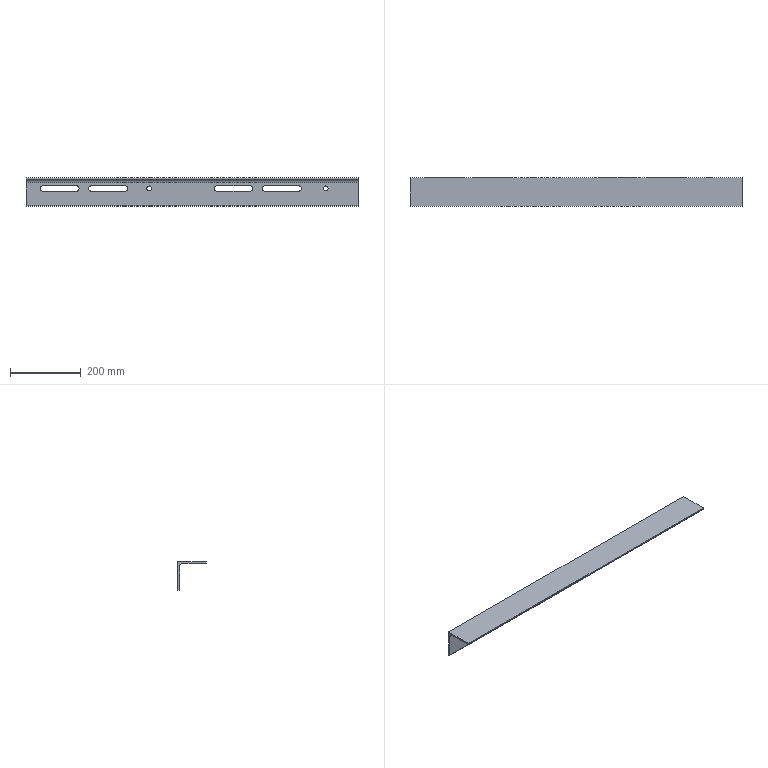Part | STEP file | Produce dryer frame-6_Default<As Machined> | 1 solid | 31 faces | box 940 x 80 x 80 mm | volume 709111 mm3 | plane 16 | cylinder 15 | commonest cylinder face diameters 15.5 x8 14 x4 3.333 x2 18 x1
STEP:
#1=CARTESIAN_POINT('',(348.5,-5.,-37.));
#2=VERTEX_POINT('',#1);
#3=CARTESIAN_POINT('',(348.5,-5.,-23.));
#4=VERTEX_POINT('',#3);
#5=CARTESIAN_POINT('',(348.5,-5.,-30.));
#6=DIRECTION('',(0.,1.,0.));
#7=DIRECTION('',(0.,0.,1.));
#8=AXIS2_PLACEMENT_3D('',#5,#6,#7);
#9=CIRCLE('',#8,7.);
#10=EDGE_CURVE('',#2,#4,#9,.T.);
#11=ORIENTED_EDGE('',*,*,#10,.F.);
#12=CARTESIAN_POINT('',(348.5,0.,-37.));
#13=VERTEX_POINT('',#12);
#14=CARTESIAN_POINT('',(348.5,0.,-37.));
#15=DIRECTION('',(0.,1.,0.));
#16=VECTOR('',#15,1000.);
#17=LINE('',#14,#16);
#18=EDGE_CURVE('',#2,#13,#17,.T.);
#19=ORIENTED_EDGE('',*,*,#18,.T.);
#20=CARTESIAN_POINT('',(348.5,0.,-23.));
#21=VERTEX_POINT('',#20);
#22=CARTESIAN_POINT('',(348.5,0.,-30.));
#23=DIRECTION('',(0.,1.,0.));
#24=DIRECTION('',(0.,0.,1.));
#25=AXIS2_PLACEMENT_3D('',#22,#23,#24);
#26=CIRCLE('',#25,7.);
#27=EDGE_CURVE('',#13,#21,#26,.T.);
#28=ORIENTED_EDGE('',*,*,#27,.T.);
#29=CARTESIAN_POINT('',(348.5,0.,-23.));
#30=DIRECTION('',(0.,1.,0.));
#31=VECTOR('',#30,1000.);
#32=LINE('',#29,#31);
#33=EDGE_CURVE('',#4,#21,#32,.T.);
#34=ORIENTED_EDGE('',*,*,#33,.F.);
#35=EDGE_LOOP('',(#11,#19,#28,#34));
#36=FACE_OUTER_BOUND('',#35,.T.);
#37=CARTESIAN_POINT('',(348.5,0.,-30.));
#38=DIRECTION('',(0.,1.,0.));
#39=DIRECTION('',(0.,0.,1.));
#40=AXIS2_PLACEMENT_3D('',#37,#38,#39);
#41=CYLINDRICAL_SURFACE('',#40,7.);
#42=ADVANCED_FACE('',(#36),#41,.F.);
#43=CARTESIAN_POINT('',(848.5,-5.,-37.));
#44=VERTEX_POINT('',#43);
#45=CARTESIAN_POINT('',(848.5,-5.,-23.));
#46=VERTEX_POINT('',#45);
#47=CARTESIAN_POINT('',(848.5,-5.,-30.));
#48=DIRECTION('',(0.,1.,0.));
#49=DIRECTION('',(0.,0.,1.));
#50=AXIS2_PLACEMENT_3D('',#47,#48,#49);
#51=CIRCLE('',#50,7.);
#52=EDGE_CURVE('',#44,#46,#51,.T.);
#53=ORIENTED_EDGE('',*,*,#52,.F.);
#54=CARTESIAN_POINT('',(848.5,0.,-37.));
#55=VERTEX_POINT('',#54);
#56=CARTESIAN_POINT('',(848.5,0.,-37.));
#57=DIRECTION('',(0.,1.,0.));
#58=VECTOR('',#57,1000.);
#59=LINE('',#56,#58);
#60=EDGE_CURVE('',#44,#55,#59,.T.);
#61=ORIENTED_EDGE('',*,*,#60,.T.);
#62=CARTESIAN_POINT('',(848.5,0.,-23.));
#63=VERTEX_POINT('',#62);
#64=CARTESIAN_POINT('',(848.5,0.,-30.));
#65=DIRECTION('',(0.,1.,0.));
#66=DIRECTION('',(0.,0.,1.));
#67=AXIS2_PLACEMENT_3D('',#64,#65,#66);
#68=CIRCLE('',#67,7.);
#69=EDGE_CURVE('',#55,#63,#68,.T.);
#70=ORIENTED_EDGE('',*,*,#69,.T.);
#71=CARTESIAN_POINT('',(848.5,0.,-23.));
#72=DIRECTION('',(0.,1.,0.));
#73=VECTOR('',#72,1000.);
#74=LINE('',#71,#73);
#75=EDGE_CURVE('',#46,#63,#74,.T.);
#76=ORIENTED_EDGE('',*,*,#75,.F.);
#77=EDGE_LOOP('',(#53,#61,#70,#76));
#78=FACE_OUTER_BOUND('',#77,.T.);
#79=CARTESIAN_POINT('',(848.5,0.,-30.));
#80=DIRECTION('',(0.,1.,0.));
#81=DIRECTION('',(0.,0.,1.));
#82=AXIS2_PLACEMENT_3D('',#79,#80,#81);
#83=CYLINDRICAL_SURFACE('',#82,7.);
#84=ADVANCED_FACE('',(#78),#83,.F.);
#85=CARTESIAN_POINT('',(848.5,0.,-30.));
#86=DIRECTION('',(0.,1.,0.));
#87=DIRECTION('',(0.,0.,1.));
#88=AXIS2_PLACEMENT_3D('',#85,#86,#87);
#89=CIRCLE('',#88,7.);
#90=EDGE_CURVE('',#63,#55,#89,.T.);
#91=ORIENTED_EDGE('',*,*,#90,.F.);
#92=ORIENTED_EDGE('',*,*,#69,.F.);
#93=EDGE_LOOP('',(#91,#92));
#94=FACE_BOUND('',#93,.T.);
#95=CARTESIAN_POINT('',(48.25,0.,-37.75));
#96=VERTEX_POINT('',#95);
#97=CARTESIAN_POINT('',(48.25,0.,-22.25));
#98=VERTEX_POINT('',#97);
#99=CARTESIAN_POINT('',(48.25,0.,-30.));
#100=DIRECTION('',(0.,1.,0.));
#101=DIRECTION('',(0.,0.,1.));
#102=AXIS2_PLACEMENT_3D('',#99,#100,#101);
#103=CIRCLE('',#102,7.75);
#104=EDGE_CURVE('',#96,#98,#103,.T.);
#105=ORIENTED_EDGE('',*,*,#104,.F.);
#106=CARTESIAN_POINT('',(142.75,0.,-37.75));
#107=VERTEX_POINT('',#106);
#108=CARTESIAN_POINT('',(142.75,0.,-37.75));
#109=DIRECTION('',(-1.,0.,0.));
#110=VECTOR('',#109,1000.);
#111=LINE('',#108,#110);
#112=EDGE_CURVE('',#107,#96,#111,.T.);
#113=ORIENTED_EDGE('',*,*,#112,.F.);
#114=CARTESIAN_POINT('',(142.75,0.,-22.25));
#115=VERTEX_POINT('',#114);
#116=CARTESIAN_POINT('',(142.75,0.,-30.));
#117=DIRECTION('',(0.,1.,0.));
#118=DIRECTION('',(0.,0.,1.));
#119=AXIS2_PLACEMENT_3D('',#116,#117,#118);
#120=CIRCLE('',#119,7.75);
#121=EDGE_CURVE('',#115,#107,#120,.T.);
#122=ORIENTED_EDGE('',*,*,#121,.F.);
#123=CARTESIAN_POINT('',(142.75,0.,-22.25));
#124=DIRECTION('',(-1.,0.,0.));
#125=VECTOR('',#124,1000.);
#126=LINE('',#123,#125);
#127=EDGE_CURVE('',#115,#98,#126,.T.);
#128=ORIENTED_EDGE('',*,*,#127,.T.);
#129=EDGE_LOOP('',(#105,#113,#122,#128));
#130=FACE_BOUND('',#129,.T.);
#131=CARTESIAN_POINT('',(279.75,0.,-37.75));
#132=VERTEX_POINT('',#131);
#133=CARTESIAN_POINT('',(185.25,0.,-37.75));
#134=VERTEX_POINT('',#133);
#135=CARTESIAN_POINT('',(279.75,0.,-37.75));
#136=DIRECTION('',(-1.,0.,0.));
#137=VECTOR('',#136,1000.);
#138=LINE('',#135,#137);
#139=EDGE_CURVE('',#132,#134,#138,.T.);
#140=ORIENTED_EDGE('',*,*,#139,.F.);
#141=CARTESIAN_POINT('',(279.75,0.,-22.25));
#142=VERTEX_POINT('',#141);
#143=CARTESIAN_POINT('',(279.75,0.,-30.));
#144=DIRECTION('',(0.,1.,0.));
#145=DIRECTION('',(0.,0.,1.));
#146=AXIS2_PLACEMENT_3D('',#143,#144,#145);
#147=CIRCLE('',#146,7.75);
#148=EDGE_CURVE('',#142,#132,#147,.T.);
#149=ORIENTED_EDGE('',*,*,#148,.F.);
#150=CARTESIAN_POINT('',(185.25,0.,-22.25));
#151=VERTEX_POINT('',#150);
#152=CARTESIAN_POINT('',(279.75,0.,-22.25));
#153=DIRECTION('',(-1.,0.,0.));
#154=VECTOR('',#153,1000.);
#155=LINE('',#152,#154);
#156=EDGE_CURVE('',#142,#151,#155,.T.);
#157=ORIENTED_EDGE('',*,*,#156,.T.);
#158=CARTESIAN_POINT('',(185.25,0.,-30.));
#159=DIRECTION('',(0.,1.,0.));
#160=DIRECTION('',(0.,0.,1.));
#161=AXIS2_PLACEMENT_3D('',#158,#159,#160);
#162=CIRCLE('',#161,7.75);
#163=EDGE_CURVE('',#134,#151,#162,.T.);
#164=ORIENTED_EDGE('',*,*,#163,.F.);
#165=EDGE_LOOP('',(#140,#149,#157,#164));
#166=FACE_BOUND('',#165,.T.);
#167=CARTESIAN_POINT('',(634.75,0.,-22.25));
#168=VERTEX_POINT('',#167);
#169=CARTESIAN_POINT('',(634.75,0.,-37.75));
#170=VERTEX_POINT('',#169);
#171=CARTESIAN_POINT('',(634.75,0.,-30.));
#172=DIRECTION('',(0.,1.,0.));
#173=DIRECTION('',(0.,0.,1.));
#174=AXIS2_PLACEMENT_3D('',#171,#172,#173);
#175=CIRCLE('',#174,7.75);
#176=EDGE_CURVE('',#168,#170,#175,.T.);
#177=ORIENTED_EDGE('',*,*,#176,.F.);
#178=CARTESIAN_POINT('',(540.25,0.,-22.25));
#179=VERTEX_POINT('',#178);
#180=CARTESIAN_POINT('',(634.75,0.,-22.25));
#181=DIRECTION('',(-1.,0.,0.));
#182=VECTOR('',#181,1000.);
#183=LINE('',#180,#182);
#184=EDGE_CURVE('',#168,#179,#183,.T.);
#185=ORIENTED_EDGE('',*,*,#184,.T.);
#186=CARTESIAN_POINT('',(540.25,0.,-37.75));
#187=VERTEX_POINT('',#186);
#188=CARTESIAN_POINT('',(540.25,0.,-30.));
#189=DIRECTION('',(0.,1.,0.));
#190=DIRECTION('',(0.,0.,1.));
#191=AXIS2_PLACEMENT_3D('',#188,#189,#190);
#192=CIRCLE('',#191,7.75);
#193=EDGE_CURVE('',#187,#179,#192,.T.);
#194=ORIENTED_EDGE('',*,*,#193,.F.);
#195=CARTESIAN_POINT('',(634.75,0.,-37.75));
#196=DIRECTION('',(-1.,0.,0.));
#197=VECTOR('',#196,1000.);
#198=LINE('',#195,#197);
#199=EDGE_CURVE('',#170,#187,#198,.T.);
#200=ORIENTED_EDGE('',*,*,#199,.F.);
#201=EDGE_LOOP('',(#177,#185,#194,#200));
#202=FACE_BOUND('',#201,.T.);
#203=CARTESIAN_POINT('',(771.75,0.,-37.75));
#204=VERTEX_POINT('',#203);
#205=CARTESIAN_POINT('',(677.25,0.,-37.75));
#206=VERTEX_POINT('',#205);
#207=CARTESIAN_POINT('',(771.75,0.,-37.75));
#208=DIRECTION('',(-1.,0.,0.));
#209=VECTOR('',#208,1000.);
#210=LINE('',#207,#209);
#211=EDGE_CURVE('',#204,#206,#210,.T.);
#212=ORIENTED_EDGE('',*,*,#211,.F.);
#213=CARTESIAN_POINT('',(771.75,0.,-22.25));
#214=VERTEX_POINT('',#213);
#215=CARTESIAN_POINT('',(771.75,0.,-30.));
#216=DIRECTION('',(0.,1.,0.));
#217=DIRECTION('',(0.,0.,1.));
#218=AXIS2_PLACEMENT_3D('',#215,#216,#217);
#219=CIRCLE('',#218,7.75);
#220=EDGE_CURVE('',#214,#204,#219,.T.);
#221=ORIENTED_EDGE('',*,*,#220,.F.);
#222=CARTESIAN_POINT('',(677.25,0.,-22.25));
#223=VERTEX_POINT('',#222);
#224=CARTESIAN_POINT('',(771.75,0.,-22.25));
#225=DIRECTION('',(-1.,0.,0.));
#226=VECTOR('',#225,1000.);
#227=LINE('',#224,#226);
#228=EDGE_CURVE('',#214,#223,#227,.T.);
#229=ORIENTED_EDGE('',*,*,#228,.T.);
#230=CARTESIAN_POINT('',(677.25,0.,-30.));
#231=DIRECTION('',(0.,1.,0.));
#232=DIRECTION('',(0.,0.,1.));
#233=AXIS2_PLACEMENT_3D('',#230,#231,#232);
#234=CIRCLE('',#233,7.75);
#235=EDGE_CURVE('',#206,#223,#234,.T.);
#236=ORIENTED_EDGE('',*,*,#235,.F.);
#237=EDGE_LOOP('',(#212,#221,#229,#236));
#238=FACE_BOUND('',#237,.T.);
#239=CARTESIAN_POINT('',(0.,0.,-80.));
#240=VERTEX_POINT('',#239);
#241=CARTESIAN_POINT('',(0.,0.,0.));
#242=VERTEX_POINT('',#241);
#243=CARTESIAN_POINT('',(0.,0.,-80.));
#244=DIRECTION('',(0.,0.,1.));
#245=VECTOR('',#244,1000.);
#246=LINE('',#243,#245);
#247=EDGE_CURVE('',#240,#242,#246,.T.);
#248=ORIENTED_EDGE('',*,*,#247,.T.);
#249=CARTESIAN_POINT('',(940.,0.,0.));
#250=VERTEX_POINT('',#249);
#251=CARTESIAN_POINT('',(940.,0.,0.));
#252=DIRECTION('',(-1.,0.,0.));
#253=VECTOR('',#252,1000.);
#254=LINE('',#251,#253);
#255=EDGE_CURVE('',#250,#242,#254,.T.);
#256=ORIENTED_EDGE('',*,*,#255,.F.);
#257=CARTESIAN_POINT('',(940.,0.,-80.));
#258=VERTEX_POINT('',#257);
#259=CARTESIAN_POINT('',(940.,0.,-80.));
#260=DIRECTION('',(0.,0.,1.));
#261=VECTOR('',#260,1000.);
#262=LINE('',#259,#261);
#263=EDGE_CURVE('',#258,#250,#262,.T.);
#264=ORIENTED_EDGE('',*,*,#263,.F.);
#265=CARTESIAN_POINT('',(940.,0.,-80.));
#266=DIRECTION('',(-1.,0.,0.));
#267=VECTOR('',#266,1000.);
#268=LINE('',#265,#267);
#269=EDGE_CURVE('',#258,#240,#268,.T.);
#270=ORIENTED_EDGE('',*,*,#269,.T.);
#271=EDGE_LOOP('',(#248,#256,#264,#270));
#272=FACE_OUTER_BOUND('',#271,.T.);
#273=CARTESIAN_POINT('',(348.5,0.,-30.));
#274=DIRECTION('',(0.,1.,0.));
#275=DIRECTION('',(0.,0.,1.));
#276=AXIS2_PLACEMENT_3D('',#273,#274,#275);
#277=CIRCLE('',#276,7.);
#278=EDGE_CURVE('',#21,#13,#277,.T.);
#279=ORIENTED_EDGE('',*,*,#278,.F.);
#280=ORIENTED_EDGE('',*,*,#27,.F.);
#281=EDGE_LOOP('',(#279,#280));
#282=FACE_BOUND('',#281,.T.);
#283=CARTESIAN_POINT('',(940.,0.,-80.));
#284=DIRECTION('',(0.,-1.,0.));
#285=DIRECTION('',(0.,0.,-1.));
#286=AXIS2_PLACEMENT_3D('',#283,#284,#285);
#287=PLANE('',#286);
#288=ADVANCED_FACE('',(#94,#130,#166,#202,#238,#272,#282),#287,.F.);
#289=CARTESIAN_POINT('',(0.,-3.333,-80.));
#290=VERTEX_POINT('',#289);
#291=CARTESIAN_POINT('',(0.,0.,-80.));
#292=DIRECTION('',(0.,1.,0.));
#293=VECTOR('',#292,1000.);
#294=LINE('',#291,#293);
#295=EDGE_CURVE('',#290,#240,#294,.T.);
#296=ORIENTED_EDGE('',*,*,#295,.T.);
#297=ORIENTED_EDGE('',*,*,#269,.F.);
#298=CARTESIAN_POINT('',(940.,-3.333,-80.));
#299=VERTEX_POINT('',#298);
#300=CARTESIAN_POINT('',(940.,0.,-80.));
#301=DIRECTION('',(0.,1.,0.));
#302=VECTOR('',#301,1000.);
#303=LINE('',#300,#302);
#304=EDGE_CURVE('',#299,#258,#303,.T.);
#305=ORIENTED_EDGE('',*,*,#304,.F.);
#306=CARTESIAN_POINT('',(940.,-3.333,-80.));
#307=DIRECTION('',(-1.,0.,0.));
#308=VECTOR('',#307,1000.);
#309=LINE('',#306,#308);
#310=EDGE_CURVE('',#299,#290,#309,.T.);
#311=ORIENTED_EDGE('',*,*,#310,.T.);
#312=EDGE_LOOP('',(#296,#297,#305,#311));
#313=FACE_OUTER_BOUND('',#312,.T.);
#314=CARTESIAN_POINT('',(940.,0.,-80.));
#315=DIRECTION('',(0.,0.,1.));
#316=DIRECTION('',(1.,0.,0.));
#317=AXIS2_PLACEMENT_3D('',#314,#315,#316);
#318=PLANE('',#317);
#319=ADVANCED_FACE('',(#313),#318,.F.);
#320=CARTESIAN_POINT('',(0.,-80.,0.));
#321=VERTEX_POINT('',#320);
#322=CARTESIAN_POINT('',(0.,0.,0.));
#323=DIRECTION('',(0.,-1.,0.));
#324=VECTOR('',#323,1000.);
#325=LINE('',#322,#324);
#326=EDGE_CURVE('',#242,#321,#325,.T.);
#327=ORIENTED_EDGE('',*,*,#326,.T.);
#328=CARTESIAN_POINT('',(940.,-80.,0.));
#329=VERTEX_POINT('',#328);
#330=CARTESIAN_POINT('',(940.,-80.,0.));
#331=DIRECTION('',(-1.,0.,0.));
#332=VECTOR('',#331,1000.);
#333=LINE('',#330,#332);
#334=EDGE_CURVE('',#329,#321,#333,.T.);
#335=ORIENTED_EDGE('',*,*,#334,.F.);
#336=CARTESIAN_POINT('',(940.,0.,0.));
#337=DIRECTION('',(0.,-1.,0.));
#338=VECTOR('',#337,1000.);
#339=LINE('',#336,#338);
#340=EDGE_CURVE('',#250,#329,#339,.T.);
#341=ORIENTED_EDGE('',*,*,#340,.F.);
#342=ORIENTED_EDGE('',*,*,#255,.T.);
#343=EDGE_LOOP('',(#327,#335,#341,#342));
#344=FACE_OUTER_BOUND('',#343,.T.);
#345=CARTESIAN_POINT('',(940.,0.,0.));
#346=DIRECTION('',(0.,0.,-1.));
#347=DIRECTION('',(0.,1.,0.));
#348=AXIS2_PLACEMENT_3D('',#345,#346,#347);
#349=PLANE('',#348);
#350=ADVANCED_FACE('',(#344),#349,.F.);
#351=CARTESIAN_POINT('',(0.,-80.,-3.333));
#352=VERTEX_POINT('',#351);
#353=CARTESIAN_POINT('',(0.,-80.,0.));
#354=DIRECTION('',(0.,0.,-1.));
#355=VECTOR('',#354,1000.);
#356=LINE('',#353,#355);
#357=EDGE_CURVE('',#321,#352,#356,.T.);
#358=ORIENTED_EDGE('',*,*,#357,.T.);
#359=CARTESIAN_POINT('',(940.,-80.,-3.333));
#360=VERTEX_POINT('',#359);
#361=CARTESIAN_POINT('',(940.,-80.,-3.333));
#362=DIRECTION('',(-1.,0.,0.));
#363=VECTOR('',#362,1000.);
#364=LINE('',#361,#363);
#365=EDGE_CURVE('',#360,#352,#364,.T.);
#366=ORIENTED_EDGE('',*,*,#365,.F.);
#367=CARTESIAN_POINT('',(940.,-80.,0.));
#368=DIRECTION('',(0.,0.,-1.));
#369=VECTOR('',#368,1000.);
#370=LINE('',#367,#369);
#371=EDGE_CURVE('',#329,#360,#370,.T.);
#372=ORIENTED_EDGE('',*,*,#371,.F.);
#373=ORIENTED_EDGE('',*,*,#334,.T.);
#374=EDGE_LOOP('',(#358,#366,#372,#373));
#375=FACE_OUTER_BOUND('',#374,.T.);
#376=CARTESIAN_POINT('',(940.,-80.,0.));
#377=DIRECTION('',(0.,1.,0.));
#378=DIRECTION('',(0.,0.,1.));
#379=AXIS2_PLACEMENT_3D('',#376,#377,#378);
#380=PLANE('',#379);
#381=ADVANCED_FACE('',(#375),#380,.F.);
#382=CARTESIAN_POINT('',(0.,-78.333,-5.));
#383=VERTEX_POINT('',#382);
#384=CARTESIAN_POINT('',(0.,-78.333,-3.333));
#385=DIRECTION('',(1.,0.,0.));
#386=DIRECTION('',(0.,0.,-1.));
#387=AXIS2_PLACEMENT_3D('',#384,#385,#386);
#388=CIRCLE('',#387,1.667);
#389=EDGE_CURVE('',#352,#383,#388,.T.);
#390=ORIENTED_EDGE('',*,*,#389,.T.);
#391=CARTESIAN_POINT('',(940.,-78.333,-5.));
#392=VERTEX_POINT('',#391);
#393=CARTESIAN_POINT('',(940.,-78.333,-5.));
#394=DIRECTION('',(-1.,0.,0.));
#395=VECTOR('',#394,1000.);
#396=LINE('',#393,#395);
#397=EDGE_CURVE('',#392,#383,#396,.T.);
#398=ORIENTED_EDGE('',*,*,#397,.F.);
#399=CARTESIAN_POINT('',(940.,-78.333,-3.333));
#400=DIRECTION('',(1.,0.,0.));
#401=DIRECTION('',(0.,0.,-1.));
#402=AXIS2_PLACEMENT_3D('',#399,#400,#401);
#403=CIRCLE('',#402,1.667);
#404=EDGE_CURVE('',#360,#392,#403,.T.);
#405=ORIENTED_EDGE('',*,*,#404,.F.);
#406=ORIENTED_EDGE('',*,*,#365,.T.);
#407=EDGE_LOOP('',(#390,#398,#405,#406));
#408=FACE_OUTER_BOUND('',#407,.T.);
#409=CARTESIAN_POINT('',(940.,-78.333,-3.333));
#410=DIRECTION('',(-1.,0.,0.));
#411=DIRECTION('',(0.,0.,1.));
#412=AXIS2_PLACEMENT_3D('',#409,#410,#411);
#413=CYLINDRICAL_SURFACE('',#412,1.667);
#414=ADVANCED_FACE('',(#408),#413,.T.);
#415=CARTESIAN_POINT('',(0.,-14.,-5.));
#416=VERTEX_POINT('',#415);
#417=CARTESIAN_POINT('',(0.,-14.,-5.));
#418=DIRECTION('',(0.,1.,0.));
#419=VECTOR('',#418,1000.);
#420=LINE('',#417,#419);
#421=EDGE_CURVE('',#383,#416,#420,.T.);
#422=ORIENTED_EDGE('',*,*,#421,.T.);
#423=CARTESIAN_POINT('',(940.,-14.,-5.));
#424=VERTEX_POINT('',#423);
#425=CARTESIAN_POINT('',(940.,-14.,-5.));
#426=DIRECTION('',(-1.,0.,0.));
#427=VECTOR('',#426,1000.);
#428=LINE('',#425,#427);
#429=EDGE_CURVE('',#424,#416,#428,.T.);
#430=ORIENTED_EDGE('',*,*,#429,.F.);
#431=CARTESIAN_POINT('',(940.,-14.,-5.));
#432=DIRECTION('',(0.,1.,0.));
#433=VECTOR('',#432,1000.);
#434=LINE('',#431,#433);
#435=EDGE_CURVE('',#392,#424,#434,.T.);
#436=ORIENTED_EDGE('',*,*,#435,.F.);
#437=ORIENTED_EDGE('',*,*,#397,.T.);
#438=EDGE_LOOP('',(#422,#430,#436,#437));
#439=FACE_OUTER_BOUND('',#438,.T.);
#440=CARTESIAN_POINT('',(940.,-14.,-5.));
#441=DIRECTION('',(0.,0.,1.));
#442=DIRECTION('',(0.,-1.,0.));
#443=AXIS2_PLACEMENT_3D('',#440,#441,#442);
#444=PLANE('',#443);
#445=ADVANCED_FACE('',(#439),#444,.F.);
#446=CARTESIAN_POINT('',(0.,-5.,-14.));
#447=VERTEX_POINT('',#446);
#448=CARTESIAN_POINT('',(0.,-14.,-14.));
#449=DIRECTION('',(-1.,0.,0.));
#450=DIRECTION('',(0.,0.,-1.));
#451=AXIS2_PLACEMENT_3D('',#448,#449,#450);
#452=CIRCLE('',#451,9.);
#453=EDGE_CURVE('',#416,#447,#452,.T.);
#454=ORIENTED_EDGE('',*,*,#453,.T.);
#455=CARTESIAN_POINT('',(940.,-5.,-14.));
#456=VERTEX_POINT('',#455);
#457=CARTESIAN_POINT('',(940.,-5.,-14.));
#458=DIRECTION('',(-1.,0.,0.));
#459=VECTOR('',#458,1000.);
#460=LINE('',#457,#459);
#461=EDGE_CURVE('',#456,#447,#460,.T.);
#462=ORIENTED_EDGE('',*,*,#461,.F.);
#463=CARTESIAN_POINT('',(940.,-14.,-14.));
#464=DIRECTION('',(-1.,0.,0.));
#465=DIRECTION('',(0.,0.,-1.));
#466=AXIS2_PLACEMENT_3D('',#463,#464,#465);
#467=CIRCLE('',#466,9.);
#468=EDGE_CURVE('',#424,#456,#467,.T.);
#469=ORIENTED_EDGE('',*,*,#468,.F.);
#470=ORIENTED_EDGE('',*,*,#429,.T.);
#471=EDGE_LOOP('',(#454,#462,#469,#470));
#472=FACE_OUTER_BOUND('',#471,.T.);
#473=CARTESIAN_POINT('',(940.,-14.,-14.));
#474=DIRECTION('',(-1.,0.,0.));
#475=DIRECTION('',(0.,0.,1.));
#476=AXIS2_PLACEMENT_3D('',#473,#474,#475);
#477=CYLINDRICAL_SURFACE('',#476,9.);
#478=ADVANCED_FACE('',(#472),#477,.F.);
#479=CARTESIAN_POINT('',(348.5,-5.,-30.));
#480=DIRECTION('',(0.,1.,0.));
#481=DIRECTION('',(0.,0.,1.));
#482=AXIS2_PLACEMENT_3D('',#479,#480,#481);
#483=CIRCLE('',#482,7.);
#484=EDGE_CURVE('',#4,#2,#483,.T.);
#485=ORIENTED_EDGE('',*,*,#484,.T.);
#486=ORIENTED_EDGE('',*,*,#10,.T.);
#487=EDGE_LOOP('',(#485,#486));
#488=FACE_BOUND('',#487,.T.);
#489=CARTESIAN_POINT('',(848.5,-5.,-30.));
#490=DIRECTION('',(0.,1.,0.));
#491=DIRECTION('',(0.,0.,1.));
#492=AXIS2_PLACEMENT_3D('',#489,#490,#491);
#493=CIRCLE('',#492,7.);
#494=EDGE_CURVE('',#46,#44,#493,.T.);
#495=ORIENTED_EDGE('',*,*,#494,.T.);
#496=ORIENTED_EDGE('',*,*,#52,.T.);
#497=EDGE_LOOP('',(#495,#496));
#498=FACE_BOUND('',#497,.T.);
#499=CARTESIAN_POINT('',(48.25,-5.,-22.25));
#500=VERTEX_POINT('',#499);
#501=CARTESIAN_POINT('',(142.75,-5.,-22.25));
#502=VERTEX_POINT('',#501);
#503=CARTESIAN_POINT('',(940.,-5.,-22.25));
#504=DIRECTION('',(1.,0.,0.));
#505=VECTOR('',#504,1000.);
#506=LINE('',#503,#505);
#507=EDGE_CURVE('',#500,#502,#506,.T.);
#508=ORIENTED_EDGE('',*,*,#507,.T.);
#509=CARTESIAN_POINT('',(142.75,-5.,-37.75));
#510=VERTEX_POINT('',#509);
#511=CARTESIAN_POINT('',(142.75,-5.,-30.));
#512=DIRECTION('',(0.,1.,0.));
#513=DIRECTION('',(0.,0.,1.));
#514=AXIS2_PLACEMENT_3D('',#511,#512,#513);
#515=CIRCLE('',#514,7.75);
#516=EDGE_CURVE('',#502,#510,#515,.T.);
#517=ORIENTED_EDGE('',*,*,#516,.T.);
#518=CARTESIAN_POINT('',(48.25,-5.,-37.75));
#519=VERTEX_POINT('',#518);
#520=CARTESIAN_POINT('',(940.,-5.,-37.75));
#521=DIRECTION('',(-1.,0.,0.));
#522=VECTOR('',#521,1000.);
#523=LINE('',#520,#522);
#524=EDGE_CURVE('',#510,#519,#523,.T.);
#525=ORIENTED_EDGE('',*,*,#524,.T.);
#526=CARTESIAN_POINT('',(48.25,-5.,-30.));
#527=DIRECTION('',(0.,1.,0.));
#528=DIRECTION('',(0.,0.,1.));
#529=AXIS2_PLACEMENT_3D('',#526,#527,#528);
#530=CIRCLE('',#529,7.75);
#531=EDGE_CURVE('',#519,#500,#530,.T.);
#532=ORIENTED_EDGE('',*,*,#531,.T.);
#533=EDGE_LOOP('',(#508,#517,#525,#532));
#534=FACE_BOUND('',#533,.T.);
#535=CARTESIAN_POINT('',(279.75,-5.,-22.25));
#536=VERTEX_POINT('',#535);
#537=CARTESIAN_POINT('',(279.75,-5.,-37.75));
#538=VERTEX_POINT('',#537);
#539=CARTESIAN_POINT('',(279.75,-5.,-30.));
#540=DIRECTION('',(0.,1.,0.));
#541=DIRECTION('',(0.,0.,1.));
#542=AXIS2_PLACEMENT_3D('',#539,#540,#541);
#543=CIRCLE('',#542,7.75);
#544=EDGE_CURVE('',#536,#538,#543,.T.);
#545=ORIENTED_EDGE('',*,*,#544,.T.);
#546=CARTESIAN_POINT('',(185.25,-5.,-37.75));
#547=VERTEX_POINT('',#546);
#548=CARTESIAN_POINT('',(940.,-5.,-37.75));
#549=DIRECTION('',(-1.,0.,0.));
#550=VECTOR('',#549,1000.);
#551=LINE('',#548,#550);
#552=EDGE_CURVE('',#538,#547,#551,.T.);
#553=ORIENTED_EDGE('',*,*,#552,.T.);
#554=CARTESIAN_POINT('',(185.25,-5.,-22.25));
#555=VERTEX_POINT('',#554);
#556=CARTESIAN_POINT('',(185.25,-5.,-30.));
#557=DIRECTION('',(0.,1.,0.));
#558=DIRECTION('',(0.,0.,1.));
#559=AXIS2_PLACEMENT_3D('',#556,#557,#558);
#560=CIRCLE('',#559,7.75);
#561=EDGE_CURVE('',#547,#555,#560,.T.);
#562=ORIENTED_EDGE('',*,*,#561,.T.);
#563=CARTESIAN_POINT('',(940.,-5.,-22.25));
#564=DIRECTION('',(1.,0.,0.));
#565=VECTOR('',#564,1000.);
#566=LINE('',#563,#565);
#567=EDGE_CURVE('',#555,#536,#566,.T.);
#568=ORIENTED_EDGE('',*,*,#567,.T.);
#569=EDGE_LOOP('',(#545,#553,#562,#568));
#570=FACE_BOUND('',#569,.T.);
#571=CARTESIAN_POINT('',(540.25,-5.,-22.25));
#572=VERTEX_POINT('',#571);
#573=CARTESIAN_POINT('',(634.75,-5.,-22.25));
#574=VERTEX_POINT('',#573);
#575=CARTESIAN_POINT('',(940.,-5.,-22.25));
#576=DIRECTION('',(1.,0.,0.));
#577=VECTOR('',#576,1000.);
#578=LINE('',#575,#577);
#579=EDGE_CURVE('',#572,#574,#578,.T.);
#580=ORIENTED_EDGE('',*,*,#579,.T.);
#581=CARTESIAN_POINT('',(634.75,-5.,-37.75));
#582=VERTEX_POINT('',#581);
#583=CARTESIAN_POINT('',(634.75,-5.,-30.));
#584=DIRECTION('',(0.,1.,0.));
#585=DIRECTION('',(0.,0.,1.));
#586=AXIS2_PLACEMENT_3D('',#583,#584,#585);
#587=CIRCLE('',#586,7.75);
#588=EDGE_CURVE('',#574,#582,#587,.T.);
#589=ORIENTED_EDGE('',*,*,#588,.T.);
#590=CARTESIAN_POINT('',(540.25,-5.,-37.75));
#591=VERTEX_POINT('',#590);
#592=CARTESIAN_POINT('',(940.,-5.,-37.75));
#593=DIRECTION('',(-1.,0.,0.));
#594=VECTOR('',#593,1000.);
#595=LINE('',#592,#594);
#596=EDGE_CURVE('',#582,#591,#595,.T.);
#597=ORIENTED_EDGE('',*,*,#596,.T.);
#598=CARTESIAN_POINT('',(540.25,-5.,-30.));
#599=DIRECTION('',(0.,1.,0.));
#600=DIRECTION('',(0.,0.,1.));
#601=AXIS2_PLACEMENT_3D('',#598,#599,#600);
#602=CIRCLE('',#601,7.75);
#603=EDGE_CURVE('',#591,#572,#602,.T.);
#604=ORIENTED_EDGE('',*,*,#603,.T.);
#605=EDGE_LOOP('',(#580,#589,#597,#604));
#606=FACE_BOUND('',#605,.T.);
#607=CARTESIAN_POINT('',(677.25,-5.,-37.75));
#608=VERTEX_POINT('',#607);
#609=CARTESIAN_POINT('',(677.25,-5.,-22.25));
#610=VERTEX_POINT('',#609);
#611=CARTESIAN_POINT('',(677.25,-5.,-30.));
#612=DIRECTION('',(0.,1.,0.));
#613=DIRECTION('',(0.,0.,1.));
#614=AXIS2_PLACEMENT_3D('',#611,#612,#613);
#615=CIRCLE('',#614,7.75);
#616=EDGE_CURVE('',#608,#610,#615,.T.);
#617=ORIENTED_EDGE('',*,*,#616,.T.);
#618=CARTESIAN_POINT('',(771.75,-5.,-22.25));
#619=VERTEX_POINT('',#618);
#620=CARTESIAN_POINT('',(940.,-5.,-22.25));
#621=DIRECTION('',(1.,0.,0.));
#622=VECTOR('',#621,1000.);
#623=LINE('',#620,#622);
#624=EDGE_CURVE('',#610,#619,#623,.T.);
#625=ORIENTED_EDGE('',*,*,#624,.T.);
#626=CARTESIAN_POINT('',(771.75,-5.,-37.75));
#627=VERTEX_POINT('',#626);
#628=CARTESIAN_POINT('',(771.75,-5.,-30.));
#629=DIRECTION('',(0.,1.,0.));
#630=DIRECTION('',(0.,0.,1.));
#631=AXIS2_PLACEMENT_3D('',#628,#629,#630);
#632=CIRCLE('',#631,7.75);
#633=EDGE_CURVE('',#619,#627,#632,.T.);
#634=ORIENTED_EDGE('',*,*,#633,.T.);
#635=CARTESIAN_POINT('',(940.,-5.,-37.75));
#636=DIRECTION('',(-1.,0.,0.));
#637=VECTOR('',#636,1000.);
#638=LINE('',#635,#637);
#639=EDGE_CURVE('',#627,#608,#638,.T.);
#640=ORIENTED_EDGE('',*,*,#639,.T.);
#641=EDGE_LOOP('',(#617,#625,#634,#640));
#642=FACE_BOUND('',#641,.T.);
#643=CARTESIAN_POINT('',(0.,-5.,-78.333));
#644=VERTEX_POINT('',#643);
#645=CARTESIAN_POINT('',(0.,-5.,-78.333));
#646=DIRECTION('',(0.,0.,-1.));
#647=VECTOR('',#646,1000.);
#648=LINE('',#645,#647);
#649=EDGE_CURVE('',#447,#644,#648,.T.);
#650=ORIENTED_EDGE('',*,*,#649,.T.);
#651=CARTESIAN_POINT('',(940.,-5.,-78.333));
#652=VERTEX_POINT('',#651);
#653=CARTESIAN_POINT('',(940.,-5.,-78.333));
#654=DIRECTION('',(-1.,0.,0.));
#655=VECTOR('',#654,1000.);
#656=LINE('',#653,#655);
#657=EDGE_CURVE('',#652,#644,#656,.T.);
#658=ORIENTED_EDGE('',*,*,#657,.F.);
#659=CARTESIAN_POINT('',(940.,-5.,-78.333));
#660=DIRECTION('',(0.,0.,-1.));
#661=VECTOR('',#660,1000.);
#662=LINE('',#659,#661);
#663=EDGE_CURVE('',#456,#652,#662,.T.);
#664=ORIENTED_EDGE('',*,*,#663,.F.);
#665=ORIENTED_EDGE('',*,*,#461,.T.);
#666=EDGE_LOOP('',(#650,#658,#664,#665));
#667=FACE_OUTER_BOUND('',#666,.T.);
#668=CARTESIAN_POINT('',(940.,-5.,-78.333));
#669=DIRECTION('',(0.,1.,0.));
#670=DIRECTION('',(0.,0.,1.));
#671=AXIS2_PLACEMENT_3D('',#668,#669,#670);
#672=PLANE('',#671);
#673=ADVANCED_FACE('',(#488,#498,#534,#570,#606,#642,#667),#672,.F.);
#674=CARTESIAN_POINT('',(0.,-3.333,-78.333));
#675=DIRECTION('',(1.,0.,0.));
#676=DIRECTION('',(0.,0.,1.));
#677=AXIS2_PLACEMENT_3D('',#674,#675,#676);
#678=CIRCLE('',#677,1.667);
#679=EDGE_CURVE('',#644,#290,#678,.T.);
#680=ORIENTED_EDGE('',*,*,#679,.T.);
#681=ORIENTED_EDGE('',*,*,#310,.F.);
#682=CARTESIAN_POINT('',(940.,-3.333,-78.333));
#683=DIRECTION('',(1.,0.,0.));
#684=DIRECTION('',(0.,0.,1.));
#685=AXIS2_PLACEMENT_3D('',#682,#683,#684);
#686=CIRCLE('',#685,1.667);
#687=EDGE_CURVE('',#652,#299,#686,.T.);
#688=ORIENTED_EDGE('',*,*,#687,.F.);
#689=ORIENTED_EDGE('',*,*,#657,.T.);
#690=EDGE_LOOP('',(#680,#681,#688,#689));
#691=FACE_OUTER_BOUND('',#690,.T.);
#692=CARTESIAN_POINT('',(940.,-3.333,-78.333));
#693=DIRECTION('',(-1.,0.,0.));
#694=DIRECTION('',(0.,0.,1.));
#695=AXIS2_PLACEMENT_3D('',#692,#693,#694);
#696=CYLINDRICAL_SURFACE('',#695,1.667);
#697=ADVANCED_FACE('',(#691),#696,.T.);
#698=ORIENTED_EDGE('',*,*,#304,.T.);
#699=ORIENTED_EDGE('',*,*,#263,.T.);
#700=ORIENTED_EDGE('',*,*,#340,.T.);
#701=ORIENTED_EDGE('',*,*,#371,.T.);
#702=ORIENTED_EDGE('',*,*,#404,.T.);
#703=ORIENTED_EDGE('',*,*,#435,.T.);
#704=ORIENTED_EDGE('',*,*,#468,.T.);
#705=ORIENTED_EDGE('',*,*,#663,.T.);
#706=ORIENTED_EDGE('',*,*,#687,.T.);
#707=EDGE_LOOP('',(#698,#699,#700,#701,#702,#703,#704,#705,#706));
#708=FACE_OUTER_BOUND('',#707,.T.);
#709=CARTESIAN_POINT('',(940.,-3.333,-78.333));
#710=DIRECTION('',(-1.,0.,0.));
#711=DIRECTION('',(0.,0.,1.));
#712=AXIS2_PLACEMENT_3D('',#709,#710,#711);
#713=PLANE('',#712);
#714=ADVANCED_FACE('',(#708),#713,.F.);
#715=ORIENTED_EDGE('',*,*,#295,.F.);
#716=ORIENTED_EDGE('',*,*,#679,.F.);
#717=ORIENTED_EDGE('',*,*,#649,.F.);
#718=ORIENTED_EDGE('',*,*,#453,.F.);
#719=ORIENTED_EDGE('',*,*,#421,.F.);
#720=ORIENTED_EDGE('',*,*,#389,.F.);
#721=ORIENTED_EDGE('',*,*,#357,.F.);
#722=ORIENTED_EDGE('',*,*,#326,.F.);
#723=ORIENTED_EDGE('',*,*,#247,.F.);
#724=EDGE_LOOP('',(#715,#716,#717,#718,#719,#720,#721,#722,#723));
#725=FACE_OUTER_BOUND('',#724,.T.);
#726=CARTESIAN_POINT('',(0.,-3.333,-78.333));
#727=DIRECTION('',(-1.,0.,0.));
#728=DIRECTION('',(0.,0.,1.));
#729=AXIS2_PLACEMENT_3D('',#726,#727,#728);
#730=PLANE('',#729);
#731=ADVANCED_FACE('',(#725),#730,.T.);
#732=CARTESIAN_POINT('',(677.25,0.,-37.75));
#733=DIRECTION('',(0.,-1.,0.));
#734=VECTOR('',#733,1000.);
#735=LINE('',#732,#734);
#736=EDGE_CURVE('',#206,#608,#735,.T.);
#737=ORIENTED_EDGE('',*,*,#736,.F.);
#738=ORIENTED_EDGE('',*,*,#235,.T.);
#739=CARTESIAN_POINT('',(677.25,0.,-22.25));
#740=DIRECTION('',(0.,1.,0.));
#741=VECTOR('',#740,1000.);
#742=LINE('',#739,#741);
#743=EDGE_CURVE('',#610,#223,#742,.T.);
#744=ORIENTED_EDGE('',*,*,#743,.F.);
#745=ORIENTED_EDGE('',*,*,#616,.F.);
#746=EDGE_LOOP('',(#737,#738,#744,#745));
#747=FACE_OUTER_BOUND('',#746,.T.);
#748=CARTESIAN_POINT('',(677.25,0.,-30.));
#749=DIRECTION('',(0.,1.,0.));
#750=DIRECTION('',(0.,0.,1.));
#751=AXIS2_PLACEMENT_3D('',#748,#749,#750);
#752=CYLINDRICAL_SURFACE('',#751,7.75);
#753=ADVANCED_FACE('',(#747),#752,.F.);
#754=CARTESIAN_POINT('',(771.75,0.,-22.25));
#755=DIRECTION('',(0.,-1.,0.));
#756=VECTOR('',#755,1000.);
#757=LINE('',#754,#756);
#758=EDGE_CURVE('',#214,#619,#757,.T.);
#759=ORIENTED_EDGE('',*,*,#758,.F.);
#760=ORIENTED_EDGE('',*,*,#220,.T.);
#761=CARTESIAN_POINT('',(771.75,0.,-37.75));
#762=DIRECTION('',(0.,1.,0.));
#763=VECTOR('',#762,1000.);
#764=LINE('',#761,#763);
#765=EDGE_CURVE('',#627,#204,#764,.T.);
#766=ORIENTED_EDGE('',*,*,#765,.F.);
#767=ORIENTED_EDGE('',*,*,#633,.F.);
#768=EDGE_LOOP('',(#759,#760,#766,#767));
#769=FACE_OUTER_BOUND('',#768,.T.);
#770=CARTESIAN_POINT('',(771.75,0.,-30.));
#771=DIRECTION('',(0.,1.,0.));
#772=DIRECTION('',(0.,0.,1.));
#773=AXIS2_PLACEMENT_3D('',#770,#771,#772);
#774=CYLINDRICAL_SURFACE('',#773,7.75);
#775=ADVANCED_FACE('',(#769),#774,.F.);
#776=ORIENTED_EDGE('',*,*,#743,.T.);
#777=ORIENTED_EDGE('',*,*,#228,.F.);
#778=ORIENTED_EDGE('',*,*,#758,.T.);
#779=ORIENTED_EDGE('',*,*,#624,.F.);
#780=EDGE_LOOP('',(#776,#777,#778,#779));
#781=FACE_OUTER_BOUND('',#780,.T.);
#782=CARTESIAN_POINT('',(771.75,0.,-22.25));
#783=DIRECTION('',(0.,0.,1.));
#784=DIRECTION('',(1.,0.,0.));
#785=AXIS2_PLACEMENT_3D('',#782,#783,#784);
#786=PLANE('',#785);
#787=ADVANCED_FACE('',(#781),#786,.F.);
#788=ORIENTED_EDGE('',*,*,#765,.T.);
#789=ORIENTED_EDGE('',*,*,#211,.T.);
#790=ORIENTED_EDGE('',*,*,#736,.T.);
#791=ORIENTED_EDGE('',*,*,#639,.F.);
#792=EDGE_LOOP('',(#788,#789,#790,#791));
#793=FACE_OUTER_BOUND('',#792,.T.);
#794=CARTESIAN_POINT('',(771.75,0.,-37.75));
#795=DIRECTION('',(0.,0.,-1.));
#796=DIRECTION('',(-1.,0.,0.));
#797=AXIS2_PLACEMENT_3D('',#794,#795,#796);
#798=PLANE('',#797);
#799=ADVANCED_FACE('',(#793),#798,.F.);
#800=CARTESIAN_POINT('',(634.75,0.,-22.25));
#801=DIRECTION('',(0.,-1.,0.));
#802=VECTOR('',#801,1000.);
#803=LINE('',#800,#802);
#804=EDGE_CURVE('',#168,#574,#803,.T.);
#805=ORIENTED_EDGE('',*,*,#804,.F.);
#806=ORIENTED_EDGE('',*,*,#176,.T.);
#807=CARTESIAN_POINT('',(634.75,0.,-37.75));
#808=DIRECTION('',(0.,1.,0.));
#809=VECTOR('',#808,1000.);
#810=LINE('',#807,#809);
#811=EDGE_CURVE('',#582,#170,#810,.T.);
#812=ORIENTED_EDGE('',*,*,#811,.F.);
#813=ORIENTED_EDGE('',*,*,#588,.F.);
#814=EDGE_LOOP('',(#805,#806,#812,#813));
#815=FACE_OUTER_BOUND('',#814,.T.);
#816=CARTESIAN_POINT('',(634.75,0.,-30.));
#817=DIRECTION('',(0.,1.,0.));
#818=DIRECTION('',(0.,0.,1.));
#819=AXIS2_PLACEMENT_3D('',#816,#817,#818);
#820=CYLINDRICAL_SURFACE('',#819,7.75);
#821=ADVANCED_FACE('',(#815),#820,.F.);
#822=CARTESIAN_POINT('',(540.25,0.,-22.25));
#823=DIRECTION('',(0.,1.,0.));
#824=VECTOR('',#823,1000.);
#825=LINE('',#822,#824);
#826=EDGE_CURVE('',#572,#179,#825,.T.);
#827=ORIENTED_EDGE('',*,*,#826,.T.);
#828=ORIENTED_EDGE('',*,*,#184,.F.);
#829=ORIENTED_EDGE('',*,*,#804,.T.);
#830=ORIENTED_EDGE('',*,*,#579,.F.);
#831=EDGE_LOOP('',(#827,#828,#829,#830));
#832=FACE_OUTER_BOUND('',#831,.T.);
#833=CARTESIAN_POINT('',(634.75,0.,-22.25));
#834=DIRECTION('',(0.,0.,1.));
#835=DIRECTION('',(1.,0.,0.));
#836=AXIS2_PLACEMENT_3D('',#833,#834,#835);
#837=PLANE('',#836);
#838=ADVANCED_FACE('',(#832),#837,.F.);
#839=ORIENTED_EDGE('',*,*,#811,.T.);
#840=ORIENTED_EDGE('',*,*,#199,.T.);
#841=CARTESIAN_POINT('',(540.25,0.,-37.75));
#842=DIRECTION('',(0.,-1.,0.));
#843=VECTOR('',#842,1000.);
#844=LINE('',#841,#843);
#845=EDGE_CURVE('',#187,#591,#844,.T.);
#846=ORIENTED_EDGE('',*,*,#845,.T.);
#847=ORIENTED_EDGE('',*,*,#596,.F.);
#848=EDGE_LOOP('',(#839,#840,#846,#847));
#849=FACE_OUTER_BOUND('',#848,.T.);
#850=CARTESIAN_POINT('',(634.75,0.,-37.75));
#851=DIRECTION('',(0.,0.,-1.));
#852=DIRECTION('',(-1.,0.,0.));
#853=AXIS2_PLACEMENT_3D('',#850,#851,#852);
#854=PLANE('',#853);
#855=ADVANCED_FACE('',(#849),#854,.F.);
#856=ORIENTED_EDGE('',*,*,#845,.F.);
#857=ORIENTED_EDGE('',*,*,#193,.T.);
#858=ORIENTED_EDGE('',*,*,#826,.F.);
#859=ORIENTED_EDGE('',*,*,#603,.F.);
#860=EDGE_LOOP('',(#856,#857,#858,#859));
#861=FACE_OUTER_BOUND('',#860,.T.);
#862=CARTESIAN_POINT('',(540.25,0.,-30.));
#863=DIRECTION('',(0.,1.,0.));
#864=DIRECTION('',(0.,0.,1.));
#865=AXIS2_PLACEMENT_3D('',#862,#863,#864);
#866=CYLINDRICAL_SURFACE('',#865,7.75);
#867=ADVANCED_FACE('',(#861),#866,.F.);
#868=CARTESIAN_POINT('',(185.25,0.,-37.75));
#869=DIRECTION('',(0.,-1.,0.));
#870=VECTOR('',#869,1000.);
#871=LINE('',#868,#870);
#872=EDGE_CURVE('',#134,#547,#871,.T.);
#873=ORIENTED_EDGE('',*,*,#872,.F.);
#874=ORIENTED_EDGE('',*,*,#163,.T.);
#875=CARTESIAN_POINT('',(185.25,0.,-22.25));
#876=DIRECTION('',(0.,1.,0.));
#877=VECTOR('',#876,1000.);
#878=LINE('',#875,#877);
#879=EDGE_CURVE('',#555,#151,#878,.T.);
#880=ORIENTED_EDGE('',*,*,#879,.F.);
#881=ORIENTED_EDGE('',*,*,#561,.F.);
#882=EDGE_LOOP('',(#873,#874,#880,#881));
#883=FACE_OUTER_BOUND('',#882,.T.);
#884=CARTESIAN_POINT('',(185.25,0.,-30.));
#885=DIRECTION('',(0.,1.,0.));
#886=DIRECTION('',(0.,0.,1.));
#887=AXIS2_PLACEMENT_3D('',#884,#885,#886);
#888=CYLINDRICAL_SURFACE('',#887,7.75);
#889=ADVANCED_FACE('',(#883),#888,.F.);
#890=CARTESIAN_POINT('',(279.75,0.,-22.25));
#891=DIRECTION('',(0.,-1.,0.));
#892=VECTOR('',#891,1000.);
#893=LINE('',#890,#892);
#894=EDGE_CURVE('',#142,#536,#893,.T.);
#895=ORIENTED_EDGE('',*,*,#894,.F.);
#896=ORIENTED_EDGE('',*,*,#148,.T.);
#897=CARTESIAN_POINT('',(279.75,0.,-37.75));
#898=DIRECTION('',(0.,1.,0.));
#899=VECTOR('',#898,1000.);
#900=LINE('',#897,#899);
#901=EDGE_CURVE('',#538,#132,#900,.T.);
#902=ORIENTED_EDGE('',*,*,#901,.F.);
#903=ORIENTED_EDGE('',*,*,#544,.F.);
#904=EDGE_LOOP('',(#895,#896,#902,#903));
#905=FACE_OUTER_BOUND('',#904,.T.);
#906=CARTESIAN_POINT('',(279.75,0.,-30.));
#907=DIRECTION('',(0.,1.,0.));
#908=DIRECTION('',(0.,0.,1.));
#909=AXIS2_PLACEMENT_3D('',#906,#907,#908);
#910=CYLINDRICAL_SURFACE('',#909,7.75);
#911=ADVANCED_FACE('',(#905),#910,.F.);
#912=ORIENTED_EDGE('',*,*,#879,.T.);
#913=ORIENTED_EDGE('',*,*,#156,.F.);
#914=ORIENTED_EDGE('',*,*,#894,.T.);
#915=ORIENTED_EDGE('',*,*,#567,.F.);
#916=EDGE_LOOP('',(#912,#913,#914,#915));
#917=FACE_OUTER_BOUND('',#916,.T.);
#918=CARTESIAN_POINT('',(279.75,0.,-22.25));
#919=DIRECTION('',(0.,0.,1.));
#920=DIRECTION('',(1.,0.,0.));
#921=AXIS2_PLACEMENT_3D('',#918,#919,#920);
#922=PLANE('',#921);
#923=ADVANCED_FACE('',(#917),#922,.F.);
#924=ORIENTED_EDGE('',*,*,#901,.T.);
#925=ORIENTED_EDGE('',*,*,#139,.T.);
#926=ORIENTED_EDGE('',*,*,#872,.T.);
#927=ORIENTED_EDGE('',*,*,#552,.F.);
#928=EDGE_LOOP('',(#924,#925,#926,#927));
#929=FACE_OUTER_BOUND('',#928,.T.);
#930=CARTESIAN_POINT('',(279.75,0.,-37.75));
#931=DIRECTION('',(0.,0.,-1.));
#932=DIRECTION('',(-1.,0.,0.));
#933=AXIS2_PLACEMENT_3D('',#930,#931,#932);
#934=PLANE('',#933);
#935=ADVANCED_FACE('',(#929),#934,.F.);
#936=CARTESIAN_POINT('',(48.25,0.,-37.75));
#937=DIRECTION('',(0.,-1.,0.));
#938=VECTOR('',#937,1000.);
#939=LINE('',#936,#938);
#940=EDGE_CURVE('',#96,#519,#939,.T.);
#941=ORIENTED_EDGE('',*,*,#940,.F.);
#942=ORIENTED_EDGE('',*,*,#104,.T.);
#943=CARTESIAN_POINT('',(48.25,0.,-22.25));
#944=DIRECTION('',(0.,1.,0.));
#945=VECTOR('',#944,1000.);
#946=LINE('',#943,#945);
#947=EDGE_CURVE('',#500,#98,#946,.T.);
#948=ORIENTED_EDGE('',*,*,#947,.F.);
#949=ORIENTED_EDGE('',*,*,#531,.F.);
#950=EDGE_LOOP('',(#941,#942,#948,#949));
#951=FACE_OUTER_BOUND('',#950,.T.);
#952=CARTESIAN_POINT('',(48.25,0.,-30.));
#953=DIRECTION('',(0.,1.,0.));
#954=DIRECTION('',(0.,0.,1.));
#955=AXIS2_PLACEMENT_3D('',#952,#953,#954);
#956=CYLINDRICAL_SURFACE('',#955,7.75);
#957=ADVANCED_FACE('',(#951),#956,.F.);
#958=ORIENTED_EDGE('',*,*,#947,.T.);
#959=ORIENTED_EDGE('',*,*,#127,.F.);
#960=CARTESIAN_POINT('',(142.75,0.,-22.25));
#961=DIRECTION('',(0.,-1.,0.));
#962=VECTOR('',#961,1000.);
#963=LINE('',#960,#962);
#964=EDGE_CURVE('',#115,#502,#963,.T.);
#965=ORIENTED_EDGE('',*,*,#964,.T.);
#966=ORIENTED_EDGE('',*,*,#507,.F.);
#967=EDGE_LOOP('',(#958,#959,#965,#966));
#968=FACE_OUTER_BOUND('',#967,.T.);
#969=CARTESIAN_POINT('',(142.75,0.,-22.25));
#970=DIRECTION('',(0.,0.,1.));
#971=DIRECTION('',(1.,0.,0.));
#972=AXIS2_PLACEMENT_3D('',#969,#970,#971);
#973=PLANE('',#972);
#974=ADVANCED_FACE('',(#968),#973,.F.);
#975=CARTESIAN_POINT('',(142.75,0.,-37.75));
#976=DIRECTION('',(0.,1.,0.));
#977=VECTOR('',#976,1000.);
#978=LINE('',#975,#977);
#979=EDGE_CURVE('',#510,#107,#978,.T.);
#980=ORIENTED_EDGE('',*,*,#979,.T.);
#981=ORIENTED_EDGE('',*,*,#112,.T.);
#982=ORIENTED_EDGE('',*,*,#940,.T.);
#983=ORIENTED_EDGE('',*,*,#524,.F.);
#984=EDGE_LOOP('',(#980,#981,#982,#983));
#985=FACE_OUTER_BOUND('',#984,.T.);
#986=CARTESIAN_POINT('',(142.75,0.,-37.75));
#987=DIRECTION('',(0.,0.,-1.));
#988=DIRECTION('',(-1.,0.,0.));
#989=AXIS2_PLACEMENT_3D('',#986,#987,#988);
#990=PLANE('',#989);
#991=ADVANCED_FACE('',(#985),#990,.F.);
#992=ORIENTED_EDGE('',*,*,#964,.F.);
#993=ORIENTED_EDGE('',*,*,#121,.T.);
#994=ORIENTED_EDGE('',*,*,#979,.F.);
#995=ORIENTED_EDGE('',*,*,#516,.F.);
#996=EDGE_LOOP('',(#992,#993,#994,#995));
#997=FACE_OUTER_BOUND('',#996,.T.);
#998=CARTESIAN_POINT('',(142.75,0.,-30.));
#999=DIRECTION('',(0.,1.,0.));
#1000=DIRECTION('',(0.,0.,1.));
#1001=AXIS2_PLACEMENT_3D('',#998,#999,#1000);
#1002=CYLINDRICAL_SURFACE('',#1001,7.75);
#1003=ADVANCED_FACE('',(#997),#1002,.F.);
#1004=ORIENTED_EDGE('',*,*,#60,.F.);
#1005=ORIENTED_EDGE('',*,*,#494,.F.);
#1006=ORIENTED_EDGE('',*,*,#75,.T.);
#1007=ORIENTED_EDGE('',*,*,#90,.T.);
#1008=EDGE_LOOP('',(#1004,#1005,#1006,#1007));
#1009=FACE_OUTER_BOUND('',#1008,.T.);
#1010=CARTESIAN_POINT('',(848.5,0.,-30.));
#1011=DIRECTION('',(0.,1.,0.));
#1012=DIRECTION('',(0.,0.,1.));
#1013=AXIS2_PLACEMENT_3D('',#1010,#1011,#1012);
#1014=CYLINDRICAL_SURFACE('',#1013,7.);
#1015=ADVANCED_FACE('',(#1009),#1014,.F.);
#1016=ORIENTED_EDGE('',*,*,#18,.F.);
#1017=ORIENTED_EDGE('',*,*,#484,.F.);
#1018=ORIENTED_EDGE('',*,*,#33,.T.);
#1019=ORIENTED_EDGE('',*,*,#278,.T.);
#1020=EDGE_LOOP('',(#1016,#1017,#1018,#1019));
#1021=FACE_OUTER_BOUND('',#1020,.T.);
#1022=CARTESIAN_POINT('',(348.5,0.,-30.));
#1023=DIRECTION('',(0.,1.,0.));
#1024=DIRECTION('',(0.,0.,1.));
#1025=AXIS2_PLACEMENT_3D('',#1022,#1023,#1024);
#1026=CYLINDRICAL_SURFACE('',#1025,7.);
#1027=ADVANCED_FACE('',(#1021),#1026,.F.);
#1028=CLOSED_SHELL('',(#42,#84,#288,#319,#350,#381,#414,#445,#478,#673,#697,#714,#731,#753,#775,#787,#799,#821,#838,#855,#867,#889,#911,#923,#935,#957,#974,#991,#1003,#1015,#1027));
#1029=MANIFOLD_SOLID_BREP('',#1028);
#1030=CARTESIAN_POINT('',(0.,0.,0.));
#1031=DIRECTION('',(0.,0.,1.));
#1032=DIRECTION('',(1.,0.,0.));
#1033=AXIS2_PLACEMENT_3D('',#1030,#1031,#1032);
#1034=(LENGTH_UNIT()NAMED_UNIT(*)SI_UNIT(.MILLI.,.METRE.));
#1035=UNCERTAINTY_MEASURE_WITH_UNIT(LENGTH_MEASURE(0.00001),#1034,'','');
#1036=(NAMED_UNIT(*)PLANE_ANGLE_UNIT()SI_UNIT($,.RADIAN.));
#1037=(NAMED_UNIT(*)SI_UNIT($,.STERADIAN.)SOLID_ANGLE_UNIT());
#1038=(GEOMETRIC_REPRESENTATION_CONTEXT(3)GLOBAL_UNCERTAINTY_ASSIGNED_CONTEXT((#1035))GLOBAL_UNIT_ASSIGNED_CONTEXT((#1034,#1036,#1037))REPRESENTATION_CONTEXT('',''));
#1039=ADVANCED_BREP_SHAPE_REPRESENTATION('',(#1029,#1033),#1038);